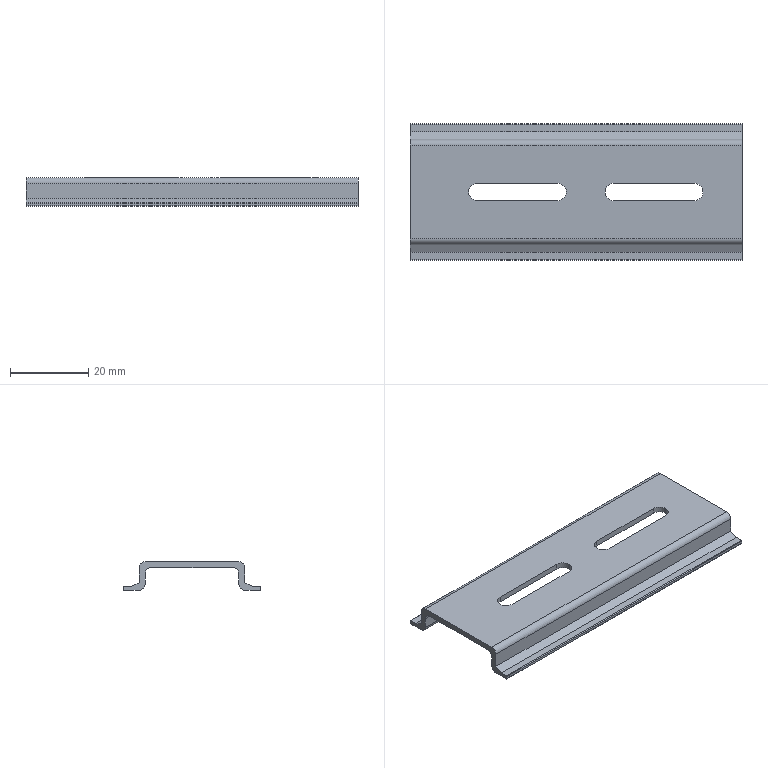Part | STEP file | MRB-85 | 1 solid | 36 faces | box 85 x 35 x 7.3 mm | volume 5359 mm3 | plane 20 | cylinder 16 | commonest cylinder face diameters 3 x6 4.5 x6 0.4 x4
STEP:
#1=CARTESIAN_POINT('',(72.75,19.75,5.8));
#2=VERTEX_POINT('',#1);
#3=CARTESIAN_POINT('',(75.,17.5,5.8));
#4=VERTEX_POINT('',#3);
#5=CARTESIAN_POINT('',(72.75,17.5,5.8));
#6=DIRECTION('',(0.,0.,-1.));
#7=DIRECTION('',(-1.,0.,0.));
#8=AXIS2_PLACEMENT_3D('',#5,#6,#7);
#9=CIRCLE('',#8,2.25);
#10=EDGE_CURVE('',#2,#4,#9,.T.);
#11=ORIENTED_EDGE('',*,*,#10,.T.);
#12=CARTESIAN_POINT('',(75.,17.5,7.3));
#13=VERTEX_POINT('',#12);
#14=CARTESIAN_POINT('',(75.,17.5,5.8));
#15=DIRECTION('',(0.,0.,1.));
#16=VECTOR('',#15,1000.);
#17=LINE('',#14,#16);
#18=EDGE_CURVE('',#4,#13,#17,.T.);
#19=ORIENTED_EDGE('',*,*,#18,.T.);
#20=CARTESIAN_POINT('',(72.75,19.75,7.3));
#21=VERTEX_POINT('',#20);
#22=CARTESIAN_POINT('',(72.75,17.5,7.3));
#23=DIRECTION('',(0.,0.,1.));
#24=DIRECTION('',(-1.,0.,0.));
#25=AXIS2_PLACEMENT_3D('',#22,#23,#24);
#26=CIRCLE('',#25,2.25);
#27=EDGE_CURVE('',#13,#21,#26,.T.);
#28=ORIENTED_EDGE('',*,*,#27,.T.);
#29=CARTESIAN_POINT('',(72.75,19.75,5.8));
#30=DIRECTION('',(0.,0.,1.));
#31=VECTOR('',#30,1000.);
#32=LINE('',#29,#31);
#33=EDGE_CURVE('',#2,#21,#32,.T.);
#34=ORIENTED_EDGE('',*,*,#33,.F.);
#35=EDGE_LOOP('',(#11,#19,#28,#34));
#36=FACE_OUTER_BOUND('',#35,.T.);
#37=CARTESIAN_POINT('',(72.75,17.5,5.8));
#38=DIRECTION('',(0.,0.,1.));
#39=DIRECTION('',(1.,0.,0.));
#40=AXIS2_PLACEMENT_3D('',#37,#38,#39);
#41=CYLINDRICAL_SURFACE('',#40,2.25);
#42=ADVANCED_FACE('',(#36),#41,.F.);
#43=CARTESIAN_POINT('',(37.75,19.75,5.8));
#44=VERTEX_POINT('',#43);
#45=CARTESIAN_POINT('',(40.,17.5,5.8));
#46=VERTEX_POINT('',#45);
#47=CARTESIAN_POINT('',(37.75,17.5,5.8));
#48=DIRECTION('',(0.,0.,-1.));
#49=DIRECTION('',(-1.,0.,0.));
#50=AXIS2_PLACEMENT_3D('',#47,#48,#49);
#51=CIRCLE('',#50,2.25);
#52=EDGE_CURVE('',#44,#46,#51,.T.);
#53=ORIENTED_EDGE('',*,*,#52,.T.);
#54=CARTESIAN_POINT('',(40.,17.5,7.3));
#55=VERTEX_POINT('',#54);
#56=CARTESIAN_POINT('',(40.,17.5,5.8));
#57=DIRECTION('',(0.,0.,1.));
#58=VECTOR('',#57,1000.);
#59=LINE('',#56,#58);
#60=EDGE_CURVE('',#46,#55,#59,.T.);
#61=ORIENTED_EDGE('',*,*,#60,.T.);
#62=CARTESIAN_POINT('',(37.75,19.75,7.3));
#63=VERTEX_POINT('',#62);
#64=CARTESIAN_POINT('',(37.75,17.5,7.3));
#65=DIRECTION('',(0.,0.,1.));
#66=DIRECTION('',(-1.,0.,0.));
#67=AXIS2_PLACEMENT_3D('',#64,#65,#66);
#68=CIRCLE('',#67,2.25);
#69=EDGE_CURVE('',#55,#63,#68,.T.);
#70=ORIENTED_EDGE('',*,*,#69,.T.);
#71=CARTESIAN_POINT('',(37.75,19.75,5.8));
#72=DIRECTION('',(0.,0.,1.));
#73=VECTOR('',#72,1000.);
#74=LINE('',#71,#73);
#75=EDGE_CURVE('',#44,#63,#74,.T.);
#76=ORIENTED_EDGE('',*,*,#75,.F.);
#77=EDGE_LOOP('',(#53,#61,#70,#76));
#78=FACE_OUTER_BOUND('',#77,.T.);
#79=CARTESIAN_POINT('',(37.75,17.5,5.8));
#80=DIRECTION('',(0.,0.,1.));
#81=DIRECTION('',(1.,0.,0.));
#82=AXIS2_PLACEMENT_3D('',#79,#80,#81);
#83=CYLINDRICAL_SURFACE('',#82,2.25);
#84=ADVANCED_FACE('',(#78),#83,.F.);
#85=CARTESIAN_POINT('',(85.,0.2,0.));
#86=VERTEX_POINT('',#85);
#87=CARTESIAN_POINT('',(85.,4.,0.));
#88=VERTEX_POINT('',#87);
#89=CARTESIAN_POINT('',(85.,0.,0.));
#90=DIRECTION('',(0.,1.,0.));
#91=VECTOR('',#90,1000.);
#92=LINE('',#89,#91);
#93=EDGE_CURVE('',#86,#88,#92,.T.);
#94=ORIENTED_EDGE('',*,*,#93,.F.);
#95=CARTESIAN_POINT('',(0.,0.2,0.));
#96=VERTEX_POINT('',#95);
#97=CARTESIAN_POINT('',(0.,0.2,0.));
#98=DIRECTION('',(1.,0.,0.));
#99=VECTOR('',#98,1000.);
#100=LINE('',#97,#99);
#101=EDGE_CURVE('',#96,#86,#100,.T.);
#102=ORIENTED_EDGE('',*,*,#101,.F.);
#103=CARTESIAN_POINT('',(0.,4.,0.));
#104=VERTEX_POINT('',#103);
#105=CARTESIAN_POINT('',(0.,4.,0.));
#106=DIRECTION('',(0.,-1.,0.));
#107=VECTOR('',#106,1000.);
#108=LINE('',#105,#107);
#109=EDGE_CURVE('',#104,#96,#108,.T.);
#110=ORIENTED_EDGE('',*,*,#109,.F.);
#111=CARTESIAN_POINT('',(0.,4.,0.));
#112=DIRECTION('',(1.,0.,0.));
#113=VECTOR('',#112,1000.);
#114=LINE('',#111,#113);
#115=EDGE_CURVE('',#104,#88,#114,.T.);
#116=ORIENTED_EDGE('',*,*,#115,.T.);
#117=EDGE_LOOP('',(#94,#102,#110,#116));
#118=FACE_OUTER_BOUND('',#117,.T.);
#119=CARTESIAN_POINT('',(0.,4.,0.));
#120=DIRECTION('',(0.,0.,1.));
#121=DIRECTION('',(1.,0.,0.));
#122=AXIS2_PLACEMENT_3D('',#119,#120,#121);
#123=PLANE('',#122);
#124=ADVANCED_FACE('',(#118),#123,.F.);
#125=CARTESIAN_POINT('',(85.,31.,0.));
#126=VERTEX_POINT('',#125);
#127=CARTESIAN_POINT('',(85.,34.8,0.));
#128=VERTEX_POINT('',#127);
#129=CARTESIAN_POINT('',(85.,0.,0.));
#130=DIRECTION('',(0.,1.,0.));
#131=VECTOR('',#130,1000.);
#132=LINE('',#129,#131);
#133=EDGE_CURVE('',#126,#128,#132,.T.);
#134=ORIENTED_EDGE('',*,*,#133,.F.);
#135=CARTESIAN_POINT('',(0.,31.,0.));
#136=VERTEX_POINT('',#135);
#137=CARTESIAN_POINT('',(0.,31.,0.));
#138=DIRECTION('',(1.,0.,0.));
#139=VECTOR('',#138,1000.);
#140=LINE('',#137,#139);
#141=EDGE_CURVE('',#136,#126,#140,.T.);
#142=ORIENTED_EDGE('',*,*,#141,.F.);
#143=CARTESIAN_POINT('',(0.,34.8,0.));
#144=VERTEX_POINT('',#143);
#145=CARTESIAN_POINT('',(0.,34.8,0.));
#146=DIRECTION('',(0.,-1.,0.));
#147=VECTOR('',#146,1000.);
#148=LINE('',#145,#147);
#149=EDGE_CURVE('',#144,#136,#148,.T.);
#150=ORIENTED_EDGE('',*,*,#149,.F.);
#151=CARTESIAN_POINT('',(0.,34.8,0.));
#152=DIRECTION('',(1.,0.,0.));
#153=VECTOR('',#152,1000.);
#154=LINE('',#151,#153);
#155=EDGE_CURVE('',#144,#128,#154,.T.);
#156=ORIENTED_EDGE('',*,*,#155,.T.);
#157=EDGE_LOOP('',(#134,#142,#150,#156));
#158=FACE_OUTER_BOUND('',#157,.T.);
#159=CARTESIAN_POINT('',(0.,34.8,0.));
#160=DIRECTION('',(0.,0.,1.));
#161=DIRECTION('',(1.,0.,0.));
#162=AXIS2_PLACEMENT_3D('',#159,#160,#161);
#163=PLANE('',#162);
#164=ADVANCED_FACE('',(#158),#163,.F.);
#165=ORIENTED_EDGE('',*,*,#101,.T.);
#166=CARTESIAN_POINT('',(85.,0.,0.2));
#167=VERTEX_POINT('',#166);
#168=CARTESIAN_POINT('',(85.,0.2,0.2));
#169=DIRECTION('',(-1.,0.,0.));
#170=DIRECTION('',(0.,0.,1.));
#171=AXIS2_PLACEMENT_3D('',#168,#169,#170);
#172=CIRCLE('',#171,0.2);
#173=EDGE_CURVE('',#86,#167,#172,.T.);
#174=ORIENTED_EDGE('',*,*,#173,.T.);
#175=CARTESIAN_POINT('',(0.,0.,0.2));
#176=VERTEX_POINT('',#175);
#177=CARTESIAN_POINT('',(0.,0.,0.2));
#178=DIRECTION('',(1.,0.,0.));
#179=VECTOR('',#178,1000.);
#180=LINE('',#177,#179);
#181=EDGE_CURVE('',#176,#167,#180,.T.);
#182=ORIENTED_EDGE('',*,*,#181,.F.);
#183=CARTESIAN_POINT('',(0.,0.2,0.2));
#184=DIRECTION('',(-1.,0.,0.));
#185=DIRECTION('',(0.,0.,1.));
#186=AXIS2_PLACEMENT_3D('',#183,#184,#185);
#187=CIRCLE('',#186,0.2);
#188=EDGE_CURVE('',#96,#176,#187,.T.);
#189=ORIENTED_EDGE('',*,*,#188,.F.);
#190=EDGE_LOOP('',(#165,#174,#182,#189));
#191=FACE_OUTER_BOUND('',#190,.T.);
#192=CARTESIAN_POINT('',(0.,0.2,0.2));
#193=DIRECTION('',(1.,0.,0.));
#194=DIRECTION('',(0.,0.,-1.));
#195=AXIS2_PLACEMENT_3D('',#192,#193,#194);
#196=CYLINDRICAL_SURFACE('',#195,0.2);
#197=ADVANCED_FACE('',(#191),#196,.T.);
#198=ORIENTED_EDGE('',*,*,#181,.T.);
#199=CARTESIAN_POINT('',(85.,0.,0.8));
#200=VERTEX_POINT('',#199);
#201=CARTESIAN_POINT('',(85.,0.,3.65));
#202=DIRECTION('',(0.,0.,1.));
#203=VECTOR('',#202,1000.);
#204=LINE('',#201,#203);
#205=EDGE_CURVE('',#167,#200,#204,.T.);
#206=ORIENTED_EDGE('',*,*,#205,.T.);
#207=CARTESIAN_POINT('',(0.,0.,0.8));
#208=VERTEX_POINT('',#207);
#209=CARTESIAN_POINT('',(0.,0.,0.8));
#210=DIRECTION('',(1.,0.,0.));
#211=VECTOR('',#210,1000.);
#212=LINE('',#209,#211);
#213=EDGE_CURVE('',#208,#200,#212,.T.);
#214=ORIENTED_EDGE('',*,*,#213,.F.);
#215=CARTESIAN_POINT('',(0.,0.,0.2));
#216=DIRECTION('',(0.,0.,1.));
#217=VECTOR('',#216,1000.);
#218=LINE('',#215,#217);
#219=EDGE_CURVE('',#176,#208,#218,.T.);
#220=ORIENTED_EDGE('',*,*,#219,.F.);
#221=EDGE_LOOP('',(#198,#206,#214,#220));
#222=FACE_OUTER_BOUND('',#221,.T.);
#223=CARTESIAN_POINT('',(0.,0.,0.2));
#224=DIRECTION('',(0.,1.,0.));
#225=DIRECTION('',(0.,0.,-1.));
#226=AXIS2_PLACEMENT_3D('',#223,#224,#225);
#227=PLANE('',#226);
#228=ADVANCED_FACE('',(#222),#227,.F.);
#229=ORIENTED_EDGE('',*,*,#213,.T.);
#230=CARTESIAN_POINT('',(85.,0.2,1.));
#231=VERTEX_POINT('',#230);
#232=CARTESIAN_POINT('',(85.,0.2,0.8));
#233=DIRECTION('',(-1.,0.,0.));
#234=DIRECTION('',(0.,0.,1.));
#235=AXIS2_PLACEMENT_3D('',#232,#233,#234);
#236=CIRCLE('',#235,0.2);
#237=EDGE_CURVE('',#200,#231,#236,.T.);
#238=ORIENTED_EDGE('',*,*,#237,.T.);
#239=CARTESIAN_POINT('',(0.,0.2,1.));
#240=VERTEX_POINT('',#239);
#241=CARTESIAN_POINT('',(0.,0.2,1.));
#242=DIRECTION('',(1.,0.,0.));
#243=VECTOR('',#242,1000.);
#244=LINE('',#241,#243);
#245=EDGE_CURVE('',#240,#231,#244,.T.);
#246=ORIENTED_EDGE('',*,*,#245,.F.);
#247=CARTESIAN_POINT('',(0.,0.2,0.8));
#248=DIRECTION('',(-1.,0.,0.));
#249=DIRECTION('',(0.,0.,1.));
#250=AXIS2_PLACEMENT_3D('',#247,#248,#249);
#251=CIRCLE('',#250,0.2);
#252=EDGE_CURVE('',#208,#240,#251,.T.);
#253=ORIENTED_EDGE('',*,*,#252,.F.);
#254=EDGE_LOOP('',(#229,#238,#246,#253));
#255=FACE_OUTER_BOUND('',#254,.T.);
#256=CARTESIAN_POINT('',(0.,0.2,0.8));
#257=DIRECTION('',(1.,0.,0.));
#258=DIRECTION('',(0.,0.,-1.));
#259=AXIS2_PLACEMENT_3D('',#256,#257,#258);
#260=CYLINDRICAL_SURFACE('',#259,0.2);
#261=ADVANCED_FACE('',(#255),#260,.T.);
#262=ORIENTED_EDGE('',*,*,#245,.T.);
#263=CARTESIAN_POINT('',(85.,2.037,1.));
#264=VERTEX_POINT('',#263);
#265=CARTESIAN_POINT('',(85.,0.2,1.));
#266=DIRECTION('',(0.,1.,0.));
#267=VECTOR('',#266,1000.);
#268=LINE('',#265,#267);
#269=EDGE_CURVE('',#231,#264,#268,.T.);
#270=ORIENTED_EDGE('',*,*,#269,.T.);
#271=CARTESIAN_POINT('',(0.,2.037,1.));
#272=VERTEX_POINT('',#271);
#273=CARTESIAN_POINT('',(0.,2.037,1.));
#274=DIRECTION('',(1.,0.,0.));
#275=VECTOR('',#274,1000.);
#276=LINE('',#273,#275);
#277=EDGE_CURVE('',#272,#264,#276,.T.);
#278=ORIENTED_EDGE('',*,*,#277,.F.);
#279=CARTESIAN_POINT('',(0.,0.2,1.));
#280=DIRECTION('',(0.,1.,0.));
#281=VECTOR('',#280,1000.);
#282=LINE('',#279,#281);
#283=EDGE_CURVE('',#240,#272,#282,.T.);
#284=ORIENTED_EDGE('',*,*,#283,.F.);
#285=EDGE_LOOP('',(#262,#270,#278,#284));
#286=FACE_OUTER_BOUND('',#285,.T.);
#287=CARTESIAN_POINT('',(0.,0.2,1.));
#288=DIRECTION('',(0.,0.,-1.));
#289=DIRECTION('',(-1.,0.,0.));
#290=AXIS2_PLACEMENT_3D('',#287,#288,#289);
#291=PLANE('',#290);
#292=ADVANCED_FACE('',(#286),#291,.F.);
#293=ORIENTED_EDGE('',*,*,#277,.T.);
#294=CARTESIAN_POINT('',(85.,4.,2.));
#295=VERTEX_POINT('',#294);
#296=CARTESIAN_POINT('',(85.,2.037,1.));
#297=DIRECTION('',(0.,0.891,0.454));
#298=VECTOR('',#297,1000.);
#299=LINE('',#296,#298);
#300=EDGE_CURVE('',#264,#295,#299,.T.);
#301=ORIENTED_EDGE('',*,*,#300,.T.);
#302=CARTESIAN_POINT('',(0.,4.,2.));
#303=VERTEX_POINT('',#302);
#304=CARTESIAN_POINT('',(0.,4.,2.));
#305=DIRECTION('',(1.,0.,0.));
#306=VECTOR('',#305,1000.);
#307=LINE('',#304,#306);
#308=EDGE_CURVE('',#303,#295,#307,.T.);
#309=ORIENTED_EDGE('',*,*,#308,.F.);
#310=CARTESIAN_POINT('',(0.,2.037,1.));
#311=DIRECTION('',(0.,0.891,0.454));
#312=VECTOR('',#311,1000.);
#313=LINE('',#310,#312);
#314=EDGE_CURVE('',#272,#303,#313,.T.);
#315=ORIENTED_EDGE('',*,*,#314,.F.);
#316=EDGE_LOOP('',(#293,#301,#309,#315));
#317=FACE_OUTER_BOUND('',#316,.T.);
#318=CARTESIAN_POINT('',(0.,2.037,1.));
#319=DIRECTION('',(0.,0.454,-0.891));
#320=DIRECTION('',(0.,-0.891,-0.454));
#321=AXIS2_PLACEMENT_3D('',#318,#319,#320);
#322=PLANE('',#321);
#323=ADVANCED_FACE('',(#317),#322,.F.);
#324=ORIENTED_EDGE('',*,*,#308,.T.);
#325=CARTESIAN_POINT('',(85.,4.,5.8));
#326=VERTEX_POINT('',#325);
#327=CARTESIAN_POINT('',(85.,4.,2.));
#328=DIRECTION('',(0.,0.,1.));
#329=VECTOR('',#328,1000.);
#330=LINE('',#327,#329);
#331=EDGE_CURVE('',#295,#326,#330,.T.);
#332=ORIENTED_EDGE('',*,*,#331,.T.);
#333=CARTESIAN_POINT('',(0.,4.,5.8));
#334=VERTEX_POINT('',#333);
#335=CARTESIAN_POINT('',(0.,4.,5.8));
#336=DIRECTION('',(1.,0.,0.));
#337=VECTOR('',#336,1000.);
#338=LINE('',#335,#337);
#339=EDGE_CURVE('',#334,#326,#338,.T.);
#340=ORIENTED_EDGE('',*,*,#339,.F.);
#341=CARTESIAN_POINT('',(0.,4.,2.));
#342=DIRECTION('',(0.,0.,1.));
#343=VECTOR('',#342,1000.);
#344=LINE('',#341,#343);
#345=EDGE_CURVE('',#303,#334,#344,.T.);
#346=ORIENTED_EDGE('',*,*,#345,.F.);
#347=EDGE_LOOP('',(#324,#332,#340,#346));
#348=FACE_OUTER_BOUND('',#347,.T.);
#349=CARTESIAN_POINT('',(0.,4.,2.));
#350=DIRECTION('',(0.,1.,0.));
#351=DIRECTION('',(0.,0.,-1.));
#352=AXIS2_PLACEMENT_3D('',#349,#350,#351);
#353=PLANE('',#352);
#354=ADVANCED_FACE('',(#348),#353,.F.);
#355=ORIENTED_EDGE('',*,*,#339,.T.);
#356=CARTESIAN_POINT('',(85.,5.5,7.3));
#357=VERTEX_POINT('',#356);
#358=CARTESIAN_POINT('',(85.,5.5,5.8));
#359=DIRECTION('',(-1.,0.,0.));
#360=DIRECTION('',(0.,0.,1.));
#361=AXIS2_PLACEMENT_3D('',#358,#359,#360);
#362=CIRCLE('',#361,1.5);
#363=EDGE_CURVE('',#326,#357,#362,.T.);
#364=ORIENTED_EDGE('',*,*,#363,.T.);
#365=CARTESIAN_POINT('',(0.,5.5,7.3));
#366=VERTEX_POINT('',#365);
#367=CARTESIAN_POINT('',(0.,5.5,7.3));
#368=DIRECTION('',(1.,0.,0.));
#369=VECTOR('',#368,1000.);
#370=LINE('',#367,#369);
#371=EDGE_CURVE('',#366,#357,#370,.T.);
#372=ORIENTED_EDGE('',*,*,#371,.F.);
#373=CARTESIAN_POINT('',(0.,5.5,5.8));
#374=DIRECTION('',(-1.,0.,0.));
#375=DIRECTION('',(0.,0.,1.));
#376=AXIS2_PLACEMENT_3D('',#373,#374,#375);
#377=CIRCLE('',#376,1.5);
#378=EDGE_CURVE('',#334,#366,#377,.T.);
#379=ORIENTED_EDGE('',*,*,#378,.F.);
#380=EDGE_LOOP('',(#355,#364,#372,#379));
#381=FACE_OUTER_BOUND('',#380,.T.);
#382=CARTESIAN_POINT('',(0.,5.5,5.8));
#383=DIRECTION('',(1.,0.,0.));
#384=DIRECTION('',(0.,0.,-1.));
#385=AXIS2_PLACEMENT_3D('',#382,#383,#384);
#386=CYLINDRICAL_SURFACE('',#385,1.5);
#387=ADVANCED_FACE('',(#381),#386,.T.);
#388=CARTESIAN_POINT('',(52.25,19.75,7.3));
#389=VERTEX_POINT('',#388);
#390=CARTESIAN_POINT('',(0.,19.75,7.3));
#391=DIRECTION('',(-1.,0.,0.));
#392=VECTOR('',#391,1000.);
#393=LINE('',#390,#392);
#394=EDGE_CURVE('',#21,#389,#393,.T.);
#395=ORIENTED_EDGE('',*,*,#394,.F.);
#396=ORIENTED_EDGE('',*,*,#27,.F.);
#397=CARTESIAN_POINT('',(72.75,15.25,7.3));
#398=VERTEX_POINT('',#397);
#399=CARTESIAN_POINT('',(72.75,17.5,7.3));
#400=DIRECTION('',(0.,0.,1.));
#401=DIRECTION('',(-1.,0.,0.));
#402=AXIS2_PLACEMENT_3D('',#399,#400,#401);
#403=CIRCLE('',#402,2.25);
#404=EDGE_CURVE('',#398,#13,#403,.T.);
#405=ORIENTED_EDGE('',*,*,#404,.F.);
#406=CARTESIAN_POINT('',(52.25,15.25,7.3));
#407=VERTEX_POINT('',#406);
#408=CARTESIAN_POINT('',(0.,15.25,7.3));
#409=DIRECTION('',(1.,0.,0.));
#410=VECTOR('',#409,1000.);
#411=LINE('',#408,#410);
#412=EDGE_CURVE('',#407,#398,#411,.T.);
#413=ORIENTED_EDGE('',*,*,#412,.F.);
#414=CARTESIAN_POINT('',(52.25,17.5,7.3));
#415=DIRECTION('',(0.,0.,1.));
#416=DIRECTION('',(-1.,0.,0.));
#417=AXIS2_PLACEMENT_3D('',#414,#415,#416);
#418=CIRCLE('',#417,2.25);
#419=EDGE_CURVE('',#389,#407,#418,.T.);
#420=ORIENTED_EDGE('',*,*,#419,.F.);
#421=EDGE_LOOP('',(#395,#396,#405,#413,#420));
#422=FACE_BOUND('',#421,.T.);
#423=ORIENTED_EDGE('',*,*,#371,.T.);
#424=CARTESIAN_POINT('',(85.,29.5,7.3));
#425=VERTEX_POINT('',#424);
#426=CARTESIAN_POINT('',(85.,0.,7.3));
#427=DIRECTION('',(0.,1.,0.));
#428=VECTOR('',#427,1000.);
#429=LINE('',#426,#428);
#430=EDGE_CURVE('',#357,#425,#429,.T.);
#431=ORIENTED_EDGE('',*,*,#430,.T.);
#432=CARTESIAN_POINT('',(0.,29.5,7.3));
#433=VERTEX_POINT('',#432);
#434=CARTESIAN_POINT('',(0.,29.5,7.3));
#435=DIRECTION('',(1.,0.,0.));
#436=VECTOR('',#435,1000.);
#437=LINE('',#434,#436);
#438=EDGE_CURVE('',#433,#425,#437,.T.);
#439=ORIENTED_EDGE('',*,*,#438,.F.);
#440=CARTESIAN_POINT('',(0.,5.5,7.3));
#441=DIRECTION('',(0.,1.,0.));
#442=VECTOR('',#441,1000.);
#443=LINE('',#440,#442);
#444=EDGE_CURVE('',#366,#433,#443,.T.);
#445=ORIENTED_EDGE('',*,*,#444,.F.);
#446=EDGE_LOOP('',(#423,#431,#439,#445));
#447=FACE_OUTER_BOUND('',#446,.T.);
#448=CARTESIAN_POINT('',(17.25,19.75,7.3));
#449=VERTEX_POINT('',#448);
#450=CARTESIAN_POINT('',(0.,19.75,7.3));
#451=DIRECTION('',(-1.,0.,0.));
#452=VECTOR('',#451,1000.);
#453=LINE('',#450,#452);
#454=EDGE_CURVE('',#63,#449,#453,.T.);
#455=ORIENTED_EDGE('',*,*,#454,.F.);
#456=ORIENTED_EDGE('',*,*,#69,.F.);
#457=CARTESIAN_POINT('',(37.75,15.25,7.3));
#458=VERTEX_POINT('',#457);
#459=CARTESIAN_POINT('',(37.75,17.5,7.3));
#460=DIRECTION('',(0.,0.,1.));
#461=DIRECTION('',(-1.,0.,0.));
#462=AXIS2_PLACEMENT_3D('',#459,#460,#461);
#463=CIRCLE('',#462,2.25);
#464=EDGE_CURVE('',#458,#55,#463,.T.);
#465=ORIENTED_EDGE('',*,*,#464,.F.);
#466=CARTESIAN_POINT('',(17.25,15.25,7.3));
#467=VERTEX_POINT('',#466);
#468=CARTESIAN_POINT('',(0.,15.25,7.3));
#469=DIRECTION('',(1.,0.,0.));
#470=VECTOR('',#469,1000.);
#471=LINE('',#468,#470);
#472=EDGE_CURVE('',#467,#458,#471,.T.);
#473=ORIENTED_EDGE('',*,*,#472,.F.);
#474=CARTESIAN_POINT('',(17.25,17.5,7.3));
#475=DIRECTION('',(0.,0.,1.));
#476=DIRECTION('',(-1.,0.,0.));
#477=AXIS2_PLACEMENT_3D('',#474,#475,#476);
#478=CIRCLE('',#477,2.25);
#479=EDGE_CURVE('',#449,#467,#478,.T.);
#480=ORIENTED_EDGE('',*,*,#479,.F.);
#481=EDGE_LOOP('',(#455,#456,#465,#473,#480));
#482=FACE_BOUND('',#481,.T.);
#483=CARTESIAN_POINT('',(0.,5.5,7.3));
#484=DIRECTION('',(0.,0.,-1.));
#485=DIRECTION('',(-1.,0.,0.));
#486=AXIS2_PLACEMENT_3D('',#483,#484,#485);
#487=PLANE('',#486);
#488=ADVANCED_FACE('',(#422,#447,#482),#487,.F.);
#489=ORIENTED_EDGE('',*,*,#438,.T.);
#490=CARTESIAN_POINT('',(85.,31.,5.8));
#491=VERTEX_POINT('',#490);
#492=CARTESIAN_POINT('',(85.,29.5,5.8));
#493=DIRECTION('',(-1.,0.,0.));
#494=DIRECTION('',(0.,0.,1.));
#495=AXIS2_PLACEMENT_3D('',#492,#493,#494);
#496=CIRCLE('',#495,1.5);
#497=EDGE_CURVE('',#425,#491,#496,.T.);
#498=ORIENTED_EDGE('',*,*,#497,.T.);
#499=CARTESIAN_POINT('',(0.,31.,5.8));
#500=VERTEX_POINT('',#499);
#501=CARTESIAN_POINT('',(0.,31.,5.8));
#502=DIRECTION('',(1.,0.,0.));
#503=VECTOR('',#502,1000.);
#504=LINE('',#501,#503);
#505=EDGE_CURVE('',#500,#491,#504,.T.);
#506=ORIENTED_EDGE('',*,*,#505,.F.);
#507=CARTESIAN_POINT('',(0.,29.5,5.8));
#508=DIRECTION('',(-1.,0.,0.));
#509=DIRECTION('',(0.,0.,1.));
#510=AXIS2_PLACEMENT_3D('',#507,#508,#509);
#511=CIRCLE('',#510,1.5);
#512=EDGE_CURVE('',#433,#500,#511,.T.);
#513=ORIENTED_EDGE('',*,*,#512,.F.);
#514=EDGE_LOOP('',(#489,#498,#506,#513));
#515=FACE_OUTER_BOUND('',#514,.T.);
#516=CARTESIAN_POINT('',(0.,29.5,5.8));
#517=DIRECTION('',(1.,0.,0.));
#518=DIRECTION('',(0.,0.,-1.));
#519=AXIS2_PLACEMENT_3D('',#516,#517,#518);
#520=CYLINDRICAL_SURFACE('',#519,1.5);
#521=ADVANCED_FACE('',(#515),#520,.T.);
#522=ORIENTED_EDGE('',*,*,#505,.T.);
#523=CARTESIAN_POINT('',(85.,31.,2.));
#524=VERTEX_POINT('',#523);
#525=CARTESIAN_POINT('',(85.,31.,5.8));
#526=DIRECTION('',(0.,0.,-1.));
#527=VECTOR('',#526,1000.);
#528=LINE('',#525,#527);
#529=EDGE_CURVE('',#491,#524,#528,.T.);
#530=ORIENTED_EDGE('',*,*,#529,.T.);
#531=CARTESIAN_POINT('',(0.,31.,2.));
#532=VERTEX_POINT('',#531);
#533=CARTESIAN_POINT('',(0.,31.,2.));
#534=DIRECTION('',(1.,0.,0.));
#535=VECTOR('',#534,1000.);
#536=LINE('',#533,#535);
#537=EDGE_CURVE('',#532,#524,#536,.T.);
#538=ORIENTED_EDGE('',*,*,#537,.F.);
#539=CARTESIAN_POINT('',(0.,31.,5.8));
#540=DIRECTION('',(0.,0.,-1.));
#541=VECTOR('',#540,1000.);
#542=LINE('',#539,#541);
#543=EDGE_CURVE('',#500,#532,#542,.T.);
#544=ORIENTED_EDGE('',*,*,#543,.F.);
#545=EDGE_LOOP('',(#522,#530,#538,#544));
#546=FACE_OUTER_BOUND('',#545,.T.);
#547=CARTESIAN_POINT('',(0.,31.,5.8));
#548=DIRECTION('',(0.,-1.,0.));
#549=DIRECTION('',(0.,0.,1.));
#550=AXIS2_PLACEMENT_3D('',#547,#548,#549);
#551=PLANE('',#550);
#552=ADVANCED_FACE('',(#546),#551,.F.);
#553=ORIENTED_EDGE('',*,*,#537,.T.);
#554=CARTESIAN_POINT('',(85.,32.963,1.));
#555=VERTEX_POINT('',#554);
#556=CARTESIAN_POINT('',(85.,31.,2.));
#557=DIRECTION('',(0.,0.891,-0.454));
#558=VECTOR('',#557,1000.);
#559=LINE('',#556,#558);
#560=EDGE_CURVE('',#524,#555,#559,.T.);
#561=ORIENTED_EDGE('',*,*,#560,.T.);
#562=CARTESIAN_POINT('',(0.,32.963,1.));
#563=VERTEX_POINT('',#562);
#564=CARTESIAN_POINT('',(0.,32.963,1.));
#565=DIRECTION('',(1.,0.,0.));
#566=VECTOR('',#565,1000.);
#567=LINE('',#564,#566);
#568=EDGE_CURVE('',#563,#555,#567,.T.);
#569=ORIENTED_EDGE('',*,*,#568,.F.);
#570=CARTESIAN_POINT('',(0.,31.,2.));
#571=DIRECTION('',(0.,0.891,-0.454));
#572=VECTOR('',#571,1000.);
#573=LINE('',#570,#572);
#574=EDGE_CURVE('',#532,#563,#573,.T.);
#575=ORIENTED_EDGE('',*,*,#574,.F.);
#576=EDGE_LOOP('',(#553,#561,#569,#575));
#577=FACE_OUTER_BOUND('',#576,.T.);
#578=CARTESIAN_POINT('',(0.,31.,2.));
#579=DIRECTION('',(0.,-0.454,-0.891));
#580=DIRECTION('',(0.,-0.891,0.454));
#581=AXIS2_PLACEMENT_3D('',#578,#579,#580);
#582=PLANE('',#581);
#583=ADVANCED_FACE('',(#577),#582,.F.);
#584=ORIENTED_EDGE('',*,*,#568,.T.);
#585=CARTESIAN_POINT('',(85.,34.8,1.));
#586=VERTEX_POINT('',#585);
#587=CARTESIAN_POINT('',(85.,32.963,1.));
#588=DIRECTION('',(0.,1.,0.));
#589=VECTOR('',#588,1000.);
#590=LINE('',#587,#589);
#591=EDGE_CURVE('',#555,#586,#590,.T.);
#592=ORIENTED_EDGE('',*,*,#591,.T.);
#593=CARTESIAN_POINT('',(0.,34.8,1.));
#594=VERTEX_POINT('',#593);
#595=CARTESIAN_POINT('',(0.,34.8,1.));
#596=DIRECTION('',(1.,0.,0.));
#597=VECTOR('',#596,1000.);
#598=LINE('',#595,#597);
#599=EDGE_CURVE('',#594,#586,#598,.T.);
#600=ORIENTED_EDGE('',*,*,#599,.F.);
#601=CARTESIAN_POINT('',(0.,32.963,1.));
#602=DIRECTION('',(0.,1.,0.));
#603=VECTOR('',#602,1000.);
#604=LINE('',#601,#603);
#605=EDGE_CURVE('',#563,#594,#604,.T.);
#606=ORIENTED_EDGE('',*,*,#605,.F.);
#607=EDGE_LOOP('',(#584,#592,#600,#606));
#608=FACE_OUTER_BOUND('',#607,.T.);
#609=CARTESIAN_POINT('',(0.,32.963,1.));
#610=DIRECTION('',(0.,0.,-1.));
#611=DIRECTION('',(-1.,0.,0.));
#612=AXIS2_PLACEMENT_3D('',#609,#610,#611);
#613=PLANE('',#612);
#614=ADVANCED_FACE('',(#608),#613,.F.);
#615=ORIENTED_EDGE('',*,*,#599,.T.);
#616=CARTESIAN_POINT('',(85.,35.,0.8));
#617=VERTEX_POINT('',#616);
#618=CARTESIAN_POINT('',(85.,34.8,0.8));
#619=DIRECTION('',(-1.,0.,0.));
#620=DIRECTION('',(0.,0.,1.));
#621=AXIS2_PLACEMENT_3D('',#618,#619,#620);
#622=CIRCLE('',#621,0.2);
#623=EDGE_CURVE('',#586,#617,#622,.T.);
#624=ORIENTED_EDGE('',*,*,#623,.T.);
#625=CARTESIAN_POINT('',(0.,35.,0.8));
#626=VERTEX_POINT('',#625);
#627=CARTESIAN_POINT('',(0.,35.,0.8));
#628=DIRECTION('',(1.,0.,0.));
#629=VECTOR('',#628,1000.);
#630=LINE('',#627,#629);
#631=EDGE_CURVE('',#626,#617,#630,.T.);
#632=ORIENTED_EDGE('',*,*,#631,.F.);
#633=CARTESIAN_POINT('',(0.,34.8,0.8));
#634=DIRECTION('',(-1.,0.,0.));
#635=DIRECTION('',(0.,0.,1.));
#636=AXIS2_PLACEMENT_3D('',#633,#634,#635);
#637=CIRCLE('',#636,0.2);
#638=EDGE_CURVE('',#594,#626,#637,.T.);
#639=ORIENTED_EDGE('',*,*,#638,.F.);
#640=EDGE_LOOP('',(#615,#624,#632,#639));
#641=FACE_OUTER_BOUND('',#640,.T.);
#642=CARTESIAN_POINT('',(0.,34.8,0.8));
#643=DIRECTION('',(1.,0.,0.));
#644=DIRECTION('',(0.,0.,-1.));
#645=AXIS2_PLACEMENT_3D('',#642,#643,#644);
#646=CYLINDRICAL_SURFACE('',#645,0.2);
#647=ADVANCED_FACE('',(#641),#646,.T.);
#648=ORIENTED_EDGE('',*,*,#631,.T.);
#649=CARTESIAN_POINT('',(85.,35.,0.2));
#650=VERTEX_POINT('',#649);
#651=CARTESIAN_POINT('',(85.,35.,3.65));
#652=DIRECTION('',(0.,0.,-1.));
#653=VECTOR('',#652,1000.);
#654=LINE('',#651,#653);
#655=EDGE_CURVE('',#617,#650,#654,.T.);
#656=ORIENTED_EDGE('',*,*,#655,.T.);
#657=CARTESIAN_POINT('',(0.,35.,0.2));
#658=VERTEX_POINT('',#657);
#659=CARTESIAN_POINT('',(0.,35.,0.2));
#660=DIRECTION('',(1.,0.,0.));
#661=VECTOR('',#660,1000.);
#662=LINE('',#659,#661);
#663=EDGE_CURVE('',#658,#650,#662,.T.);
#664=ORIENTED_EDGE('',*,*,#663,.F.);
#665=CARTESIAN_POINT('',(0.,35.,0.8));
#666=DIRECTION('',(0.,0.,-1.));
#667=VECTOR('',#666,1000.);
#668=LINE('',#665,#667);
#669=EDGE_CURVE('',#626,#658,#668,.T.);
#670=ORIENTED_EDGE('',*,*,#669,.F.);
#671=EDGE_LOOP('',(#648,#656,#664,#670));
#672=FACE_OUTER_BOUND('',#671,.T.);
#673=CARTESIAN_POINT('',(0.,35.,0.8));
#674=DIRECTION('',(0.,-1.,0.));
#675=DIRECTION('',(0.,0.,1.));
#676=AXIS2_PLACEMENT_3D('',#673,#674,#675);
#677=PLANE('',#676);
#678=ADVANCED_FACE('',(#672),#677,.F.);
#679=ORIENTED_EDGE('',*,*,#663,.T.);
#680=CARTESIAN_POINT('',(85.,34.8,0.2));
#681=DIRECTION('',(-1.,0.,0.));
#682=DIRECTION('',(0.,0.,1.));
#683=AXIS2_PLACEMENT_3D('',#680,#681,#682);
#684=CIRCLE('',#683,0.2);
#685=EDGE_CURVE('',#650,#128,#684,.T.);
#686=ORIENTED_EDGE('',*,*,#685,.T.);
#687=ORIENTED_EDGE('',*,*,#155,.F.);
#688=CARTESIAN_POINT('',(0.,34.8,0.2));
#689=DIRECTION('',(-1.,0.,0.));
#690=DIRECTION('',(0.,0.,1.));
#691=AXIS2_PLACEMENT_3D('',#688,#689,#690);
#692=CIRCLE('',#691,0.2);
#693=EDGE_CURVE('',#658,#144,#692,.T.);
#694=ORIENTED_EDGE('',*,*,#693,.F.);
#695=EDGE_LOOP('',(#679,#686,#687,#694));
#696=FACE_OUTER_BOUND('',#695,.T.);
#697=CARTESIAN_POINT('',(0.,34.8,0.2));
#698=DIRECTION('',(1.,0.,0.));
#699=DIRECTION('',(0.,0.,-1.));
#700=AXIS2_PLACEMENT_3D('',#697,#698,#699);
#701=CYLINDRICAL_SURFACE('',#700,0.2);
#702=ADVANCED_FACE('',(#696),#701,.T.);
#703=ORIENTED_EDGE('',*,*,#141,.T.);
#704=CARTESIAN_POINT('',(85.,29.5,1.5));
#705=VERTEX_POINT('',#704);
#706=CARTESIAN_POINT('',(85.,31.,1.5));
#707=DIRECTION('',(-1.,0.,0.));
#708=DIRECTION('',(0.,0.,1.));
#709=AXIS2_PLACEMENT_3D('',#706,#707,#708);
#710=CIRCLE('',#709,1.5);
#711=EDGE_CURVE('',#126,#705,#710,.T.);
#712=ORIENTED_EDGE('',*,*,#711,.T.);
#713=CARTESIAN_POINT('',(0.,29.5,1.5));
#714=VERTEX_POINT('',#713);
#715=CARTESIAN_POINT('',(0.,29.5,1.5));
#716=DIRECTION('',(1.,0.,0.));
#717=VECTOR('',#716,1000.);
#718=LINE('',#715,#717);
#719=EDGE_CURVE('',#714,#705,#718,.T.);
#720=ORIENTED_EDGE('',*,*,#719,.F.);
#721=CARTESIAN_POINT('',(0.,31.,1.5));
#722=DIRECTION('',(-1.,0.,0.));
#723=DIRECTION('',(0.,0.,1.));
#724=AXIS2_PLACEMENT_3D('',#721,#722,#723);
#725=CIRCLE('',#724,1.5);
#726=EDGE_CURVE('',#136,#714,#725,.T.);
#727=ORIENTED_EDGE('',*,*,#726,.F.);
#728=EDGE_LOOP('',(#703,#712,#720,#727));
#729=FACE_OUTER_BOUND('',#728,.T.);
#730=CARTESIAN_POINT('',(0.,31.,1.5));
#731=DIRECTION('',(1.,0.,0.));
#732=DIRECTION('',(0.,0.,-1.));
#733=AXIS2_PLACEMENT_3D('',#730,#731,#732);
#734=CYLINDRICAL_SURFACE('',#733,1.5);
#735=ADVANCED_FACE('',(#729),#734,.T.);
#736=ORIENTED_EDGE('',*,*,#719,.T.);
#737=CARTESIAN_POINT('',(85.,29.5,4.3));
#738=VERTEX_POINT('',#737);
#739=CARTESIAN_POINT('',(85.,29.5,1.5));
#740=DIRECTION('',(0.,0.,1.));
#741=VECTOR('',#740,1000.);
#742=LINE('',#739,#741);
#743=EDGE_CURVE('',#705,#738,#742,.T.);
#744=ORIENTED_EDGE('',*,*,#743,.T.);
#745=CARTESIAN_POINT('',(0.,29.5,4.3));
#746=VERTEX_POINT('',#745);
#747=CARTESIAN_POINT('',(0.,29.5,4.3));
#748=DIRECTION('',(1.,0.,0.));
#749=VECTOR('',#748,1000.);
#750=LINE('',#747,#749);
#751=EDGE_CURVE('',#746,#738,#750,.T.);
#752=ORIENTED_EDGE('',*,*,#751,.F.);
#753=CARTESIAN_POINT('',(0.,29.5,1.5));
#754=DIRECTION('',(0.,0.,1.));
#755=VECTOR('',#754,1000.);
#756=LINE('',#753,#755);
#757=EDGE_CURVE('',#714,#746,#756,.T.);
#758=ORIENTED_EDGE('',*,*,#757,.F.);
#759=EDGE_LOOP('',(#736,#744,#752,#758));
#760=FACE_OUTER_BOUND('',#759,.T.);
#761=CARTESIAN_POINT('',(0.,29.5,1.5));
#762=DIRECTION('',(0.,1.,0.));
#763=DIRECTION('',(0.,0.,-1.));
#764=AXIS2_PLACEMENT_3D('',#761,#762,#763);
#765=PLANE('',#764);
#766=ADVANCED_FACE('',(#760),#765,.F.);
#767=CARTESIAN_POINT('',(85.,28.,5.8));
#768=VERTEX_POINT('',#767);
#769=CARTESIAN_POINT('',(85.,28.,4.3));
#770=DIRECTION('',(-1.,0.,0.));
#771=DIRECTION('',(0.,0.,1.));
#772=AXIS2_PLACEMENT_3D('',#769,#770,#771);
#773=CIRCLE('',#772,1.5);
#774=EDGE_CURVE('',#768,#738,#773,.T.);
#775=ORIENTED_EDGE('',*,*,#774,.F.);
#776=CARTESIAN_POINT('',(0.,28.,5.8));
#777=VERTEX_POINT('',#776);
#778=CARTESIAN_POINT('',(0.,28.,5.8));
#779=DIRECTION('',(1.,0.,0.));
#780=VECTOR('',#779,1000.);
#781=LINE('',#778,#780);
#782=EDGE_CURVE('',#777,#768,#781,.T.);
#783=ORIENTED_EDGE('',*,*,#782,.F.);
#784=CARTESIAN_POINT('',(0.,28.,4.3));
#785=DIRECTION('',(-1.,0.,0.));
#786=DIRECTION('',(0.,0.,1.));
#787=AXIS2_PLACEMENT_3D('',#784,#785,#786);
#788=CIRCLE('',#787,1.5);
#789=EDGE_CURVE('',#777,#746,#788,.T.);
#790=ORIENTED_EDGE('',*,*,#789,.T.);
#791=ORIENTED_EDGE('',*,*,#751,.T.);
#792=EDGE_LOOP('',(#775,#783,#790,#791));
#793=FACE_OUTER_BOUND('',#792,.T.);
#794=CARTESIAN_POINT('',(0.,28.,4.3));
#795=DIRECTION('',(1.,0.,0.));
#796=DIRECTION('',(0.,0.,-1.));
#797=AXIS2_PLACEMENT_3D('',#794,#795,#796);
#798=CYLINDRICAL_SURFACE('',#797,1.5);
#799=ADVANCED_FACE('',(#793),#798,.F.);
#800=CARTESIAN_POINT('',(52.25,19.75,5.8));
#801=VERTEX_POINT('',#800);
#802=CARTESIAN_POINT('',(52.25,19.75,5.8));
#803=DIRECTION('',(1.,0.,0.));
#804=VECTOR('',#803,1000.);
#805=LINE('',#802,#804);
#806=EDGE_CURVE('',#801,#2,#805,.T.);
#807=ORIENTED_EDGE('',*,*,#806,.F.);
#808=CARTESIAN_POINT('',(52.25,15.25,5.8));
#809=VERTEX_POINT('',#808);
#810=CARTESIAN_POINT('',(52.25,17.5,5.8));
#811=DIRECTION('',(0.,0.,-1.));
#812=DIRECTION('',(-1.,0.,0.));
#813=AXIS2_PLACEMENT_3D('',#810,#811,#812);
#814=CIRCLE('',#813,2.25);
#815=EDGE_CURVE('',#809,#801,#814,.T.);
#816=ORIENTED_EDGE('',*,*,#815,.F.);
#817=CARTESIAN_POINT('',(72.75,15.25,5.8));
#818=VERTEX_POINT('',#817);
#819=CARTESIAN_POINT('',(72.75,15.25,5.8));
#820=DIRECTION('',(-1.,0.,0.));
#821=VECTOR('',#820,1000.);
#822=LINE('',#819,#821);
#823=EDGE_CURVE('',#818,#809,#822,.T.);
#824=ORIENTED_EDGE('',*,*,#823,.F.);
#825=CARTESIAN_POINT('',(72.75,17.5,5.8));
#826=DIRECTION('',(0.,0.,-1.));
#827=DIRECTION('',(-1.,0.,0.));
#828=AXIS2_PLACEMENT_3D('',#825,#826,#827);
#829=CIRCLE('',#828,2.25);
#830=EDGE_CURVE('',#4,#818,#829,.T.);
#831=ORIENTED_EDGE('',*,*,#830,.F.);
#832=ORIENTED_EDGE('',*,*,#10,.F.);
#833=EDGE_LOOP('',(#807,#816,#824,#831,#832));
#834=FACE_BOUND('',#833,.T.);
#835=ORIENTED_EDGE('',*,*,#782,.T.);
#836=CARTESIAN_POINT('',(85.,7.,5.8));
#837=VERTEX_POINT('',#836);
#838=CARTESIAN_POINT('',(85.,28.,5.8));
#839=DIRECTION('',(0.,-1.,0.));
#840=VECTOR('',#839,1000.);
#841=LINE('',#838,#840);
#842=EDGE_CURVE('',#768,#837,#841,.T.);
#843=ORIENTED_EDGE('',*,*,#842,.T.);
#844=CARTESIAN_POINT('',(0.,7.,5.8));
#845=VERTEX_POINT('',#844);
#846=CARTESIAN_POINT('',(0.,7.,5.8));
#847=DIRECTION('',(1.,0.,0.));
#848=VECTOR('',#847,1000.);
#849=LINE('',#846,#848);
#850=EDGE_CURVE('',#845,#837,#849,.T.);
#851=ORIENTED_EDGE('',*,*,#850,.F.);
#852=CARTESIAN_POINT('',(0.,28.,5.8));
#853=DIRECTION('',(0.,-1.,0.));
#854=VECTOR('',#853,1000.);
#855=LINE('',#852,#854);
#856=EDGE_CURVE('',#777,#845,#855,.T.);
#857=ORIENTED_EDGE('',*,*,#856,.F.);
#858=EDGE_LOOP('',(#835,#843,#851,#857));
#859=FACE_OUTER_BOUND('',#858,.T.);
#860=CARTESIAN_POINT('',(17.25,19.75,5.8));
#861=VERTEX_POINT('',#860);
#862=CARTESIAN_POINT('',(17.25,19.75,5.8));
#863=DIRECTION('',(1.,0.,0.));
#864=VECTOR('',#863,1000.);
#865=LINE('',#862,#864);
#866=EDGE_CURVE('',#861,#44,#865,.T.);
#867=ORIENTED_EDGE('',*,*,#866,.F.);
#868=CARTESIAN_POINT('',(17.25,15.25,5.8));
#869=VERTEX_POINT('',#868);
#870=CARTESIAN_POINT('',(17.25,17.5,5.8));
#871=DIRECTION('',(0.,0.,-1.));
#872=DIRECTION('',(-1.,0.,0.));
#873=AXIS2_PLACEMENT_3D('',#870,#871,#872);
#874=CIRCLE('',#873,2.25);
#875=EDGE_CURVE('',#869,#861,#874,.T.);
#876=ORIENTED_EDGE('',*,*,#875,.F.);
#877=CARTESIAN_POINT('',(37.75,15.25,5.8));
#878=VERTEX_POINT('',#877);
#879=CARTESIAN_POINT('',(37.75,15.25,5.8));
#880=DIRECTION('',(-1.,0.,0.));
#881=VECTOR('',#880,1000.);
#882=LINE('',#879,#881);
#883=EDGE_CURVE('',#878,#869,#882,.T.);
#884=ORIENTED_EDGE('',*,*,#883,.F.);
#885=CARTESIAN_POINT('',(37.75,17.5,5.8));
#886=DIRECTION('',(0.,0.,-1.));
#887=DIRECTION('',(-1.,0.,0.));
#888=AXIS2_PLACEMENT_3D('',#885,#886,#887);
#889=CIRCLE('',#888,2.25);
#890=EDGE_CURVE('',#46,#878,#889,.T.);
#891=ORIENTED_EDGE('',*,*,#890,.F.);
#892=ORIENTED_EDGE('',*,*,#52,.F.);
#893=EDGE_LOOP('',(#867,#876,#884,#891,#892));
#894=FACE_BOUND('',#893,.T.);
#895=CARTESIAN_POINT('',(0.,28.,5.8));
#896=DIRECTION('',(0.,0.,1.));
#897=DIRECTION('',(1.,0.,0.));
#898=AXIS2_PLACEMENT_3D('',#895,#896,#897);
#899=PLANE('',#898);
#900=ADVANCED_FACE('',(#834,#859,#894),#899,.F.);
#901=CARTESIAN_POINT('',(85.,5.5,4.3));
#902=VERTEX_POINT('',#901);
#903=CARTESIAN_POINT('',(85.,7.,4.3));
#904=DIRECTION('',(-1.,0.,0.));
#905=DIRECTION('',(0.,0.,1.));
#906=AXIS2_PLACEMENT_3D('',#903,#904,#905);
#907=CIRCLE('',#906,1.5);
#908=EDGE_CURVE('',#902,#837,#907,.T.);
#909=ORIENTED_EDGE('',*,*,#908,.F.);
#910=CARTESIAN_POINT('',(0.,5.5,4.3));
#911=VERTEX_POINT('',#910);
#912=CARTESIAN_POINT('',(0.,5.5,4.3));
#913=DIRECTION('',(1.,0.,0.));
#914=VECTOR('',#913,1000.);
#915=LINE('',#912,#914);
#916=EDGE_CURVE('',#911,#902,#915,.T.);
#917=ORIENTED_EDGE('',*,*,#916,.F.);
#918=CARTESIAN_POINT('',(0.,7.,4.3));
#919=DIRECTION('',(-1.,0.,0.));
#920=DIRECTION('',(0.,0.,1.));
#921=AXIS2_PLACEMENT_3D('',#918,#919,#920);
#922=CIRCLE('',#921,1.5);
#923=EDGE_CURVE('',#911,#845,#922,.T.);
#924=ORIENTED_EDGE('',*,*,#923,.T.);
#925=ORIENTED_EDGE('',*,*,#850,.T.);
#926=EDGE_LOOP('',(#909,#917,#924,#925));
#927=FACE_OUTER_BOUND('',#926,.T.);
#928=CARTESIAN_POINT('',(0.,7.,4.3));
#929=DIRECTION('',(1.,0.,0.));
#930=DIRECTION('',(0.,0.,-1.));
#931=AXIS2_PLACEMENT_3D('',#928,#929,#930);
#932=CYLINDRICAL_SURFACE('',#931,1.5);
#933=ADVANCED_FACE('',(#927),#932,.F.);
#934=ORIENTED_EDGE('',*,*,#916,.T.);
#935=CARTESIAN_POINT('',(85.,5.5,1.5));
#936=VERTEX_POINT('',#935);
#937=CARTESIAN_POINT('',(85.,5.5,4.3));
#938=DIRECTION('',(0.,0.,-1.));
#939=VECTOR('',#938,1000.);
#940=LINE('',#937,#939);
#941=EDGE_CURVE('',#902,#936,#940,.T.);
#942=ORIENTED_EDGE('',*,*,#941,.T.);
#943=CARTESIAN_POINT('',(0.,5.5,1.5));
#944=VERTEX_POINT('',#943);
#945=CARTESIAN_POINT('',(0.,5.5,1.5));
#946=DIRECTION('',(1.,0.,0.));
#947=VECTOR('',#946,1000.);
#948=LINE('',#945,#947);
#949=EDGE_CURVE('',#944,#936,#948,.T.);
#950=ORIENTED_EDGE('',*,*,#949,.F.);
#951=CARTESIAN_POINT('',(0.,5.5,4.3));
#952=DIRECTION('',(0.,0.,-1.));
#953=VECTOR('',#952,1000.);
#954=LINE('',#951,#953);
#955=EDGE_CURVE('',#911,#944,#954,.T.);
#956=ORIENTED_EDGE('',*,*,#955,.F.);
#957=EDGE_LOOP('',(#934,#942,#950,#956));
#958=FACE_OUTER_BOUND('',#957,.T.);
#959=CARTESIAN_POINT('',(0.,5.5,4.3));
#960=DIRECTION('',(0.,-1.,0.));
#961=DIRECTION('',(0.,0.,1.));
#962=AXIS2_PLACEMENT_3D('',#959,#960,#961);
#963=PLANE('',#962);
#964=ADVANCED_FACE('',(#958),#963,.F.);
#965=ORIENTED_EDGE('',*,*,#949,.T.);
#966=CARTESIAN_POINT('',(85.,4.,1.5));
#967=DIRECTION('',(-1.,0.,0.));
#968=DIRECTION('',(0.,0.,1.));
#969=AXIS2_PLACEMENT_3D('',#966,#967,#968);
#970=CIRCLE('',#969,1.5);
#971=EDGE_CURVE('',#936,#88,#970,.T.);
#972=ORIENTED_EDGE('',*,*,#971,.T.);
#973=ORIENTED_EDGE('',*,*,#115,.F.);
#974=CARTESIAN_POINT('',(0.,4.,1.5));
#975=DIRECTION('',(-1.,0.,0.));
#976=DIRECTION('',(0.,0.,1.));
#977=AXIS2_PLACEMENT_3D('',#974,#975,#976);
#978=CIRCLE('',#977,1.5);
#979=EDGE_CURVE('',#944,#104,#978,.T.);
#980=ORIENTED_EDGE('',*,*,#979,.F.);
#981=EDGE_LOOP('',(#965,#972,#973,#980));
#982=FACE_OUTER_BOUND('',#981,.T.);
#983=CARTESIAN_POINT('',(0.,4.,1.5));
#984=DIRECTION('',(1.,0.,0.));
#985=DIRECTION('',(0.,0.,-1.));
#986=AXIS2_PLACEMENT_3D('',#983,#984,#985);
#987=CYLINDRICAL_SURFACE('',#986,1.5);
#988=ADVANCED_FACE('',(#982),#987,.T.);
#989=ORIENTED_EDGE('',*,*,#109,.T.);
#990=ORIENTED_EDGE('',*,*,#188,.T.);
#991=ORIENTED_EDGE('',*,*,#219,.T.);
#992=ORIENTED_EDGE('',*,*,#252,.T.);
#993=ORIENTED_EDGE('',*,*,#283,.T.);
#994=ORIENTED_EDGE('',*,*,#314,.T.);
#995=ORIENTED_EDGE('',*,*,#345,.T.);
#996=ORIENTED_EDGE('',*,*,#378,.T.);
#997=ORIENTED_EDGE('',*,*,#444,.T.);
#998=ORIENTED_EDGE('',*,*,#512,.T.);
#999=ORIENTED_EDGE('',*,*,#543,.T.);
#1000=ORIENTED_EDGE('',*,*,#574,.T.);
#1001=ORIENTED_EDGE('',*,*,#605,.T.);
#1002=ORIENTED_EDGE('',*,*,#638,.T.);
#1003=ORIENTED_EDGE('',*,*,#669,.T.);
#1004=ORIENTED_EDGE('',*,*,#693,.T.);
#1005=ORIENTED_EDGE('',*,*,#149,.T.);
#1006=ORIENTED_EDGE('',*,*,#726,.T.);
#1007=ORIENTED_EDGE('',*,*,#757,.T.);
#1008=ORIENTED_EDGE('',*,*,#789,.F.);
#1009=ORIENTED_EDGE('',*,*,#856,.T.);
#1010=ORIENTED_EDGE('',*,*,#923,.F.);
#1011=ORIENTED_EDGE('',*,*,#955,.T.);
#1012=ORIENTED_EDGE('',*,*,#979,.T.);
#1013=EDGE_LOOP('',(#989,#990,#991,#992,#993,#994,#995,#996,#997,#998,#999,#1000,#1001,#1002,#1003,#1004,#1005,#1006,#1007,#1008,#1009,#1010,#1011,#1012));
#1014=FACE_OUTER_BOUND('',#1013,.T.);
#1015=CARTESIAN_POINT('',(0.,0.2,0.2));
#1016=DIRECTION('',(-1.,0.,0.));
#1017=DIRECTION('',(0.,0.,1.));
#1018=AXIS2_PLACEMENT_3D('',#1015,#1016,#1017);
#1019=PLANE('',#1018);
#1020=ADVANCED_FACE('',(#1014),#1019,.T.);
#1021=ORIENTED_EDGE('',*,*,#454,.T.);
#1022=CARTESIAN_POINT('',(17.25,19.75,5.8));
#1023=DIRECTION('',(0.,0.,1.));
#1024=VECTOR('',#1023,1000.);
#1025=LINE('',#1022,#1024);
#1026=EDGE_CURVE('',#861,#449,#1025,.T.);
#1027=ORIENTED_EDGE('',*,*,#1026,.F.);
#1028=ORIENTED_EDGE('',*,*,#866,.T.);
#1029=ORIENTED_EDGE('',*,*,#75,.T.);
#1030=EDGE_LOOP('',(#1021,#1027,#1028,#1029));
#1031=FACE_OUTER_BOUND('',#1030,.T.);
#1032=CARTESIAN_POINT('',(17.25,19.75,5.8));
#1033=DIRECTION('',(0.,-1.,0.));
#1034=DIRECTION('',(0.,0.,1.));
#1035=AXIS2_PLACEMENT_3D('',#1032,#1033,#1034);
#1036=PLANE('',#1035);
#1037=ADVANCED_FACE('',(#1031),#1036,.T.);
#1038=ORIENTED_EDGE('',*,*,#60,.F.);
#1039=ORIENTED_EDGE('',*,*,#890,.T.);
#1040=CARTESIAN_POINT('',(37.75,15.25,5.8));
#1041=DIRECTION('',(0.,0.,1.));
#1042=VECTOR('',#1041,1000.);
#1043=LINE('',#1040,#1042);
#1044=EDGE_CURVE('',#878,#458,#1043,.T.);
#1045=ORIENTED_EDGE('',*,*,#1044,.T.);
#1046=ORIENTED_EDGE('',*,*,#464,.T.);
#1047=EDGE_LOOP('',(#1038,#1039,#1045,#1046));
#1048=FACE_OUTER_BOUND('',#1047,.T.);
#1049=CARTESIAN_POINT('',(37.75,17.5,5.8));
#1050=DIRECTION('',(0.,0.,1.));
#1051=DIRECTION('',(1.,0.,0.));
#1052=AXIS2_PLACEMENT_3D('',#1049,#1050,#1051);
#1053=CYLINDRICAL_SURFACE('',#1052,2.25);
#1054=ADVANCED_FACE('',(#1048),#1053,.F.);
#1055=ORIENTED_EDGE('',*,*,#472,.T.);
#1056=ORIENTED_EDGE('',*,*,#1044,.F.);
#1057=ORIENTED_EDGE('',*,*,#883,.T.);
#1058=CARTESIAN_POINT('',(17.25,15.25,5.8));
#1059=DIRECTION('',(0.,0.,1.));
#1060=VECTOR('',#1059,1000.);
#1061=LINE('',#1058,#1060);
#1062=EDGE_CURVE('',#869,#467,#1061,.T.);
#1063=ORIENTED_EDGE('',*,*,#1062,.T.);
#1064=EDGE_LOOP('',(#1055,#1056,#1057,#1063));
#1065=FACE_OUTER_BOUND('',#1064,.T.);
#1066=CARTESIAN_POINT('',(37.75,15.25,5.8));
#1067=DIRECTION('',(0.,1.,0.));
#1068=DIRECTION('',(0.,0.,-1.));
#1069=AXIS2_PLACEMENT_3D('',#1066,#1067,#1068);
#1070=PLANE('',#1069);
#1071=ADVANCED_FACE('',(#1065),#1070,.T.);
#1072=ORIENTED_EDGE('',*,*,#479,.T.);
#1073=ORIENTED_EDGE('',*,*,#1062,.F.);
#1074=ORIENTED_EDGE('',*,*,#875,.T.);
#1075=ORIENTED_EDGE('',*,*,#1026,.T.);
#1076=EDGE_LOOP('',(#1072,#1073,#1074,#1075));
#1077=FACE_OUTER_BOUND('',#1076,.T.);
#1078=CARTESIAN_POINT('',(17.25,17.5,5.8));
#1079=DIRECTION('',(0.,0.,1.));
#1080=DIRECTION('',(1.,0.,0.));
#1081=AXIS2_PLACEMENT_3D('',#1078,#1079,#1080);
#1082=CYLINDRICAL_SURFACE('',#1081,2.25);
#1083=ADVANCED_FACE('',(#1077),#1082,.F.);
#1084=ORIENTED_EDGE('',*,*,#394,.T.);
#1085=CARTESIAN_POINT('',(52.25,19.75,5.8));
#1086=DIRECTION('',(0.,0.,1.));
#1087=VECTOR('',#1086,1000.);
#1088=LINE('',#1085,#1087);
#1089=EDGE_CURVE('',#801,#389,#1088,.T.);
#1090=ORIENTED_EDGE('',*,*,#1089,.F.);
#1091=ORIENTED_EDGE('',*,*,#806,.T.);
#1092=ORIENTED_EDGE('',*,*,#33,.T.);
#1093=EDGE_LOOP('',(#1084,#1090,#1091,#1092));
#1094=FACE_OUTER_BOUND('',#1093,.T.);
#1095=CARTESIAN_POINT('',(52.25,19.75,5.8));
#1096=DIRECTION('',(0.,-1.,0.));
#1097=DIRECTION('',(0.,0.,1.));
#1098=AXIS2_PLACEMENT_3D('',#1095,#1096,#1097);
#1099=PLANE('',#1098);
#1100=ADVANCED_FACE('',(#1094),#1099,.T.);
#1101=ORIENTED_EDGE('',*,*,#18,.F.);
#1102=ORIENTED_EDGE('',*,*,#830,.T.);
#1103=CARTESIAN_POINT('',(72.75,15.25,5.8));
#1104=DIRECTION('',(0.,0.,1.));
#1105=VECTOR('',#1104,1000.);
#1106=LINE('',#1103,#1105);
#1107=EDGE_CURVE('',#818,#398,#1106,.T.);
#1108=ORIENTED_EDGE('',*,*,#1107,.T.);
#1109=ORIENTED_EDGE('',*,*,#404,.T.);
#1110=EDGE_LOOP('',(#1101,#1102,#1108,#1109));
#1111=FACE_OUTER_BOUND('',#1110,.T.);
#1112=CARTESIAN_POINT('',(72.75,17.5,5.8));
#1113=DIRECTION('',(0.,0.,1.));
#1114=DIRECTION('',(1.,0.,0.));
#1115=AXIS2_PLACEMENT_3D('',#1112,#1113,#1114);
#1116=CYLINDRICAL_SURFACE('',#1115,2.25);
#1117=ADVANCED_FACE('',(#1111),#1116,.F.);
#1118=ORIENTED_EDGE('',*,*,#412,.T.);
#1119=ORIENTED_EDGE('',*,*,#1107,.F.);
#1120=ORIENTED_EDGE('',*,*,#823,.T.);
#1121=CARTESIAN_POINT('',(52.25,15.25,5.8));
#1122=DIRECTION('',(0.,0.,1.));
#1123=VECTOR('',#1122,1000.);
#1124=LINE('',#1121,#1123);
#1125=EDGE_CURVE('',#809,#407,#1124,.T.);
#1126=ORIENTED_EDGE('',*,*,#1125,.T.);
#1127=EDGE_LOOP('',(#1118,#1119,#1120,#1126));
#1128=FACE_OUTER_BOUND('',#1127,.T.);
#1129=CARTESIAN_POINT('',(72.75,15.25,5.8));
#1130=DIRECTION('',(0.,1.,0.));
#1131=DIRECTION('',(0.,0.,-1.));
#1132=AXIS2_PLACEMENT_3D('',#1129,#1130,#1131);
#1133=PLANE('',#1132);
#1134=ADVANCED_FACE('',(#1128),#1133,.T.);
#1135=ORIENTED_EDGE('',*,*,#419,.T.);
#1136=ORIENTED_EDGE('',*,*,#1125,.F.);
#1137=ORIENTED_EDGE('',*,*,#815,.T.);
#1138=ORIENTED_EDGE('',*,*,#1089,.T.);
#1139=EDGE_LOOP('',(#1135,#1136,#1137,#1138));
#1140=FACE_OUTER_BOUND('',#1139,.T.);
#1141=CARTESIAN_POINT('',(52.25,17.5,5.8));
#1142=DIRECTION('',(0.,0.,1.));
#1143=DIRECTION('',(1.,0.,0.));
#1144=AXIS2_PLACEMENT_3D('',#1141,#1142,#1143);
#1145=CYLINDRICAL_SURFACE('',#1144,2.25);
#1146=ADVANCED_FACE('',(#1140),#1145,.F.);
#1147=ORIENTED_EDGE('',*,*,#93,.T.);
#1148=ORIENTED_EDGE('',*,*,#971,.F.);
#1149=ORIENTED_EDGE('',*,*,#941,.F.);
#1150=ORIENTED_EDGE('',*,*,#908,.T.);
#1151=ORIENTED_EDGE('',*,*,#842,.F.);
#1152=ORIENTED_EDGE('',*,*,#774,.T.);
#1153=ORIENTED_EDGE('',*,*,#743,.F.);
#1154=ORIENTED_EDGE('',*,*,#711,.F.);
#1155=ORIENTED_EDGE('',*,*,#133,.T.);
#1156=ORIENTED_EDGE('',*,*,#685,.F.);
#1157=ORIENTED_EDGE('',*,*,#655,.F.);
#1158=ORIENTED_EDGE('',*,*,#623,.F.);
#1159=ORIENTED_EDGE('',*,*,#591,.F.);
#1160=ORIENTED_EDGE('',*,*,#560,.F.);
#1161=ORIENTED_EDGE('',*,*,#529,.F.);
#1162=ORIENTED_EDGE('',*,*,#497,.F.);
#1163=ORIENTED_EDGE('',*,*,#430,.F.);
#1164=ORIENTED_EDGE('',*,*,#363,.F.);
#1165=ORIENTED_EDGE('',*,*,#331,.F.);
#1166=ORIENTED_EDGE('',*,*,#300,.F.);
#1167=ORIENTED_EDGE('',*,*,#269,.F.);
#1168=ORIENTED_EDGE('',*,*,#237,.F.);
#1169=ORIENTED_EDGE('',*,*,#205,.F.);
#1170=ORIENTED_EDGE('',*,*,#173,.F.);
#1171=EDGE_LOOP('',(#1147,#1148,#1149,#1150,#1151,#1152,#1153,#1154,#1155,#1156,#1157,#1158,#1159,#1160,#1161,#1162,#1163,#1164,#1165,#1166,#1167,#1168,#1169,#1170));
#1172=FACE_OUTER_BOUND('',#1171,.T.);
#1173=CARTESIAN_POINT('',(85.,0.,3.65));
#1174=DIRECTION('',(-1.,0.,0.));
#1175=DIRECTION('',(0.,-1.,0.));
#1176=AXIS2_PLACEMENT_3D('',#1173,#1174,#1175);
#1177=PLANE('',#1176);
#1178=ADVANCED_FACE('',(#1172),#1177,.F.);
#1179=CLOSED_SHELL('',(#42,#84,#124,#164,#197,#228,#261,#292,#323,#354,#387,#488,#521,#552,#583,#614,#647,#678,#702,#735,#766,#799,#900,#933,#964,#988,#1020,#1037,#1054,#1071,#1083,#1100,#1117,#1134,#1146,#1178));
#1180=MANIFOLD_SOLID_BREP('',#1179);
#1181=CARTESIAN_POINT('',(0.,0.,0.));
#1182=DIRECTION('',(0.,0.,1.));
#1183=DIRECTION('',(1.,0.,0.));
#1184=AXIS2_PLACEMENT_3D('',#1181,#1182,#1183);
#1185=(LENGTH_UNIT()NAMED_UNIT(*)SI_UNIT(.MILLI.,.METRE.));
#1186=UNCERTAINTY_MEASURE_WITH_UNIT(LENGTH_MEASURE(0.00001),#1185,'','');
#1187=(NAMED_UNIT(*)PLANE_ANGLE_UNIT()SI_UNIT($,.RADIAN.));
#1188=(NAMED_UNIT(*)SI_UNIT($,.STERADIAN.)SOLID_ANGLE_UNIT());
#1189=(GEOMETRIC_REPRESENTATION_CONTEXT(3)GLOBAL_UNCERTAINTY_ASSIGNED_CONTEXT((#1186))GLOBAL_UNIT_ASSIGNED_CONTEXT((#1185,#1187,#1188))REPRESENTATION_CONTEXT('',''));
#1190=ADVANCED_BREP_SHAPE_REPRESENTATION('',(#1180,#1184),#1189);